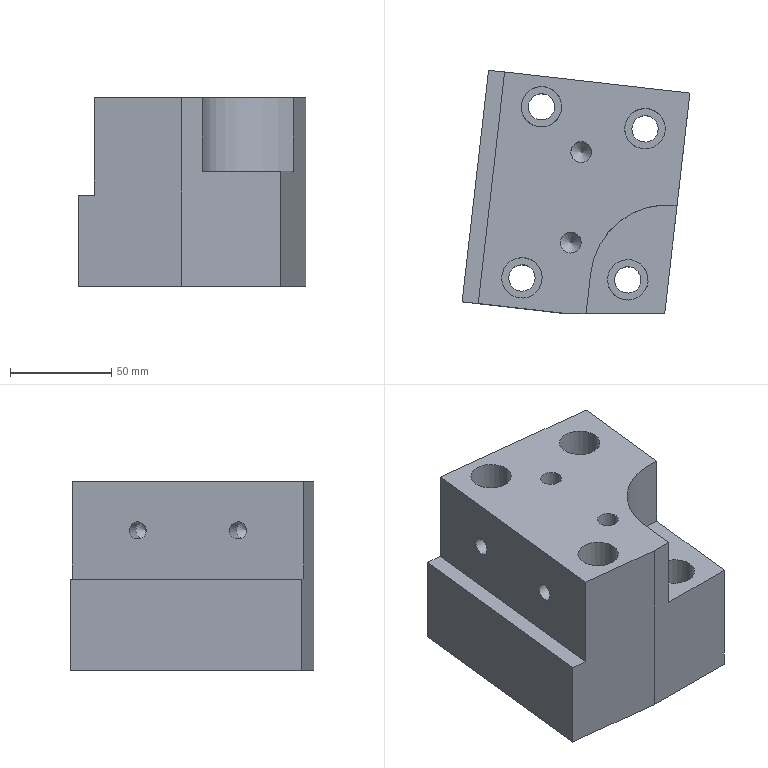Part | NX | features solid 2 | 1 solid | 32 faces | box 112.376 x 120.08 x 93 mm | volume 865745 mm3 | plane 15 | cylinder 13 | cone 4 | commonest cylinder face diameters 13 x4 20 x4 8.5 x2 10.3 x2 76 x1
STEP:
#1=CARTESIAN_POINT('',(3534.734,-298.002,-128.));
#2=VERTEX_POINT('',#1);
#3=CARTESIAN_POINT('',(3540.966,-299.848,-128.));
#4=DIRECTION('',(0.,0.,1.));
#5=DIRECTION('',(-0.9588,0.284,0.));
#6=AXIS2_PLACEMENT_3D('',#3,#4,#5);
#7=CIRCLE('',#6,6.5);
#8=EDGE_CURVE('',#2,#2,#7,.T.);
#9=ORIENTED_EDGE('',*,*,#8,.T.);
#10=EDGE_LOOP('',(#9));
#11=FACE_BOUND('',#10,.T.);
#12=CARTESIAN_POINT('',(3526.244,-372.52,-128.));
#13=VERTEX_POINT('',#12);
#14=CARTESIAN_POINT('',(3532.476,-374.366,-128.));
#15=DIRECTION('',(0.,0.,-1.));
#16=DIRECTION('',(-0.9588,0.284,0.));
#17=AXIS2_PLACEMENT_3D('',#14,#15,#16);
#18=CIRCLE('',#17,6.5);
#19=EDGE_CURVE('',#13,#13,#18,.T.);
#20=ORIENTED_EDGE('',*,*,#19,.F.);
#21=EDGE_LOOP('',(#20));
#22=FACE_BOUND('',#21,.T.);
#23=CARTESIAN_POINT('',(3474.012,-371.601,-128.));
#24=VERTEX_POINT('',#23);
#25=CARTESIAN_POINT('',(3480.244,-373.447,-128.));
#26=DIRECTION('',(0.,0.,1.));
#27=DIRECTION('',(-0.9588,0.284,0.));
#28=AXIS2_PLACEMENT_3D('',#25,#26,#27);
#29=CIRCLE('',#28,6.5);
#30=EDGE_CURVE('',#24,#24,#29,.T.);
#31=ORIENTED_EDGE('',*,*,#30,.T.);
#32=EDGE_LOOP('',(#31));
#33=FACE_BOUND('',#32,.T.);
#34=CARTESIAN_POINT('',(3483.634,-287.147,-128.));
#35=VERTEX_POINT('',#34);
#36=CARTESIAN_POINT('',(3489.867,-288.994,-128.));
#37=DIRECTION('',(0.,0.,-1.));
#38=DIRECTION('',(-0.9588,0.284,0.));
#39=AXIS2_PLACEMENT_3D('',#36,#37,#38);
#40=CIRCLE('',#39,6.5);
#41=EDGE_CURVE('',#35,#35,#40,.T.);
#42=ORIENTED_EDGE('',*,*,#41,.F.);
#43=EDGE_LOOP('',(#42));
#44=FACE_BOUND('',#43,.T.);
#45=CARTESIAN_POINT('',(3550.71,-391.,-128.));
#46=VERTEX_POINT('',#45);
#47=CARTESIAN_POINT('',(3563.102,-282.241,-128.));
#48=VERTEX_POINT('',#47);
#49=CARTESIAN_POINT('',(3549.214,-404.131,-128.));
#50=DIRECTION('',(0.1132,0.9936,0.));
#51=VECTOR('',#50,1000.);
#52=LINE('',#49,#51);
#53=EDGE_CURVE('',#46,#48,#52,.T.);
#54=ORIENTED_EDGE('',*,*,#53,.F.);
#55=CARTESIAN_POINT('',(3501.799,-391.,-128.));
#56=VERTEX_POINT('',#55);
#57=CARTESIAN_POINT('',(2433.139,-391.,-128.));
#58=DIRECTION('',(-1.,0.,0.));
#59=VECTOR('',#58,1000.);
#60=LINE('',#57,#59);
#61=EDGE_CURVE('',#46,#56,#60,.T.);
#62=ORIENTED_EDGE('',*,*,#61,.T.);
#63=CARTESIAN_POINT('',(3450.726,-385.181,-128.));
#64=VERTEX_POINT('',#63);
#65=CARTESIAN_POINT('',(3304.282,-368.496,-128.));
#66=DIRECTION('',(-0.9936,0.1132,0.));
#67=VECTOR('',#66,1000.);
#68=LINE('',#65,#67);
#69=EDGE_CURVE('',#56,#64,#68,.T.);
#70=ORIENTED_EDGE('',*,*,#69,.T.);
#71=CARTESIAN_POINT('',(3463.745,-270.92,-128.));
#72=VERTEX_POINT('',#71);
#73=CARTESIAN_POINT('',(3449.857,-392.811,-128.));
#74=DIRECTION('',(0.1132,0.9936,0.));
#75=VECTOR('',#74,1000.);
#76=LINE('',#73,#75);
#77=EDGE_CURVE('',#64,#72,#76,.T.);
#78=ORIENTED_EDGE('',*,*,#77,.T.);
#79=CARTESIAN_POINT('',(3414.066,-265.26,-128.));
#80=DIRECTION('',(0.9936,-0.1132,0.));
#81=VECTOR('',#80,1000.);
#82=LINE('',#79,#81);
#83=EDGE_CURVE('',#72,#48,#82,.T.);
#84=ORIENTED_EDGE('',*,*,#83,.T.);
#85=EDGE_LOOP('',(#54,#62,#70,#78,#84));
#86=FACE_BOUND('',#85,.T.);
#87=CARTESIAN_POINT('',(2433.139,-154.013,-128.));
#88=DIRECTION('',(0.,0.,-1.));
#89=DIRECTION('',(-0.9588,0.284,0.));
#90=AXIS2_PLACEMENT_3D('',#87,#88,#89);
#91=PLANE('',#90);
#92=ADVANCED_FACE('',(#11,#22,#33,#44,#86),#91,.T.);
#93=CARTESIAN_POINT('',(3501.799,-391.,-35.));
#94=VERTEX_POINT('',#93);
#95=CARTESIAN_POINT('',(3501.799,-391.,-118.027));
#96=DIRECTION('',(0.,0.,-1.));
#97=VECTOR('',#96,1000.);
#98=LINE('',#95,#97);
#99=EDGE_CURVE('',#94,#56,#98,.T.);
#100=ORIENTED_EDGE('',*,*,#99,.F.);
#101=CARTESIAN_POINT('',(3458.675,-386.087,-35.));
#102=VERTEX_POINT('',#101);
#103=CARTESIAN_POINT('',(3304.282,-368.496,-35.));
#104=DIRECTION('',(0.9936,-0.1132,0.));
#105=VECTOR('',#104,1000.);
#106=LINE('',#103,#105);
#107=EDGE_CURVE('',#102,#94,#106,.T.);
#108=ORIENTED_EDGE('',*,*,#107,.F.);
#109=CARTESIAN_POINT('',(3458.675,-386.087,-83.));
#110=VERTEX_POINT('',#109);
#111=CARTESIAN_POINT('',(3458.675,-386.087,-56.673));
#112=DIRECTION('',(0.,0.,1.));
#113=VECTOR('',#112,1000.);
#114=LINE('',#111,#113);
#115=EDGE_CURVE('',#110,#102,#114,.T.);
#116=ORIENTED_EDGE('',*,*,#115,.F.);
#117=CARTESIAN_POINT('',(3450.726,-385.181,-83.));
#118=VERTEX_POINT('',#117);
#119=CARTESIAN_POINT('',(3304.282,-368.496,-83.));
#120=DIRECTION('',(-0.9936,0.1132,0.));
#121=VECTOR('',#120,1000.);
#122=LINE('',#119,#121);
#123=EDGE_CURVE('',#110,#118,#122,.T.);
#124=ORIENTED_EDGE('',*,*,#123,.T.);
#125=CARTESIAN_POINT('',(3450.726,-385.181,-16.673));
#126=DIRECTION('',(0.,0.,1.));
#127=VECTOR('',#126,1000.);
#128=LINE('',#125,#127);
#129=EDGE_CURVE('',#64,#118,#128,.T.);
#130=ORIENTED_EDGE('',*,*,#129,.F.);
#131=ORIENTED_EDGE('',*,*,#69,.F.);
#132=EDGE_LOOP('',(#100,#108,#116,#124,#130,#131));
#133=FACE_BOUND('',#132,.T.);
#134=CARTESIAN_POINT('',(3304.282,-368.496,-118.027));
#135=DIRECTION('',(0.1132,0.9936,0.));
#136=DIRECTION('',(0.,0.,-1.));
#137=AXIS2_PLACEMENT_3D('',#134,#135,#136);
#138=PLANE('',#137);
#139=ADVANCED_FACE('',(#133),#138,.F.);
#140=CARTESIAN_POINT('',(3489.833,-376.287,-35.));
#141=VERTEX_POINT('',#140);
#142=CARTESIAN_POINT('',(3480.244,-373.447,-35.));
#143=DIRECTION('',(0.,0.,-1.));
#144=DIRECTION('',(0.9588,-0.284,0.));
#145=AXIS2_PLACEMENT_3D('',#142,#143,#144);
#146=CIRCLE('',#145,10.);
#147=EDGE_CURVE('',#141,#141,#146,.T.);
#148=ORIENTED_EDGE('',*,*,#147,.T.);
#149=EDGE_LOOP('',(#148));
#150=FACE_BOUND('',#149,.T.);
#151=CARTESIAN_POINT('',(3514.578,-311.938,-35.));
#152=VERTEX_POINT('',#151);
#153=CARTESIAN_POINT('',(3509.461,-311.355,-35.));
#154=DIRECTION('',(0.,0.,1.));
#155=DIRECTION('',(0.9936,-0.1132,0.));
#156=AXIS2_PLACEMENT_3D('',#153,#154,#155);
#157=CIRCLE('',#156,5.15);
#158=EDGE_CURVE('',#152,#152,#157,.T.);
#159=ORIENTED_EDGE('',*,*,#158,.F.);
#160=EDGE_LOOP('',(#159));
#161=FACE_BOUND('',#160,.T.);
#162=CARTESIAN_POINT('',(3509.484,-356.649,-35.));
#163=VERTEX_POINT('',#162);
#164=CARTESIAN_POINT('',(3504.367,-356.066,-35.));
#165=DIRECTION('',(0.,0.,1.));
#166=DIRECTION('',(0.9936,-0.1132,0.));
#167=AXIS2_PLACEMENT_3D('',#164,#165,#166);
#168=CIRCLE('',#167,5.15);
#169=EDGE_CURVE('',#163,#163,#168,.T.);
#170=ORIENTED_EDGE('',*,*,#169,.F.);
#171=EDGE_LOOP('',(#170));
#172=FACE_BOUND('',#171,.T.);
#173=CARTESIAN_POINT('',(3499.802,-290.126,-35.));
#174=VERTEX_POINT('',#173);
#175=CARTESIAN_POINT('',(3489.867,-288.994,-35.));
#176=DIRECTION('',(0.,0.,1.));
#177=DIRECTION('',(0.9936,-0.1132,0.));
#178=AXIS2_PLACEMENT_3D('',#175,#176,#177);
#179=CIRCLE('',#178,10.);
#180=EDGE_CURVE('',#174,#174,#179,.T.);
#181=ORIENTED_EDGE('',*,*,#180,.F.);
#182=EDGE_LOOP('',(#181));
#183=FACE_BOUND('',#182,.T.);
#184=CARTESIAN_POINT('',(3550.902,-300.98,-35.));
#185=VERTEX_POINT('',#184);
#186=CARTESIAN_POINT('',(3540.966,-299.848,-35.));
#187=DIRECTION('',(0.,0.,1.));
#188=DIRECTION('',(0.9936,-0.1132,0.));
#189=AXIS2_PLACEMENT_3D('',#186,#187,#188);
#190=CIRCLE('',#189,10.);
#191=EDGE_CURVE('',#185,#185,#190,.T.);
#192=ORIENTED_EDGE('',*,*,#191,.F.);
#193=EDGE_LOOP('',(#192));
#194=FACE_BOUND('',#193,.T.);
#195=ORIENTED_EDGE('',*,*,#107,.T.);
#196=CARTESIAN_POINT('',(3511.886,-391.,-35.));
#197=VERTEX_POINT('',#196);
#198=CARTESIAN_POINT('',(3507.763,-391.,-35.));
#199=DIRECTION('',(1.,0.,0.));
#200=VECTOR('',#199,1000.);
#201=LINE('',#198,#200);
#202=EDGE_CURVE('',#94,#197,#201,.T.);
#203=ORIENTED_EDGE('',*,*,#202,.T.);
#204=CARTESIAN_POINT('',(3514.147,-371.156,-35.));
#205=VERTEX_POINT('',#204);
#206=CARTESIAN_POINT('',(3519.115,-327.552,-35.));
#207=DIRECTION('',(-0.1132,-0.9936,0.));
#208=VECTOR('',#207,1000.);
#209=LINE('',#206,#208);
#210=EDGE_CURVE('',#205,#197,#209,.T.);
#211=ORIENTED_EDGE('',*,*,#210,.F.);
#212=CARTESIAN_POINT('',(3556.775,-337.771,-35.));
#213=VERTEX_POINT('',#212);
#214=CARTESIAN_POINT('',(3551.903,-375.457,-35.));
#215=DIRECTION('',(0.,0.,-1.));
#216=DIRECTION('',(0.9936,-0.1132,0.));
#217=AXIS2_PLACEMENT_3D('',#214,#215,#216);
#218=CIRCLE('',#217,38.);
#219=EDGE_CURVE('',#205,#213,#218,.T.);
#220=ORIENTED_EDGE('',*,*,#219,.T.);
#221=CARTESIAN_POINT('',(3563.102,-282.241,-35.));
#222=VERTEX_POINT('',#221);
#223=CARTESIAN_POINT('',(3549.214,-404.131,-35.));
#224=DIRECTION('',(-0.1132,-0.9936,0.));
#225=VECTOR('',#224,1000.);
#226=LINE('',#223,#225);
#227=EDGE_CURVE('',#222,#213,#226,.T.);
#228=ORIENTED_EDGE('',*,*,#227,.F.);
#229=CARTESIAN_POINT('',(3471.693,-271.826,-35.));
#230=VERTEX_POINT('',#229);
#231=CARTESIAN_POINT('',(3513.423,-276.58,-35.));
#232=DIRECTION('',(0.9936,-0.1132,0.));
#233=VECTOR('',#232,1000.);
#234=LINE('',#231,#233);
#235=EDGE_CURVE('',#230,#222,#234,.T.);
#236=ORIENTED_EDGE('',*,*,#235,.F.);
#237=CARTESIAN_POINT('',(3457.806,-393.716,-35.));
#238=DIRECTION('',(-0.1132,-0.9936,0.));
#239=VECTOR('',#238,1000.);
#240=LINE('',#237,#239);
#241=EDGE_CURVE('',#230,#102,#240,.T.);
#242=ORIENTED_EDGE('',*,*,#241,.T.);
#243=EDGE_LOOP('',(#195,#203,#211,#220,#228,#236,#242));
#244=FACE_BOUND('',#243,.T.);
#245=CARTESIAN_POINT('',(3507.763,-326.259,-35.));
#246=DIRECTION('',(0.,0.,1.));
#247=DIRECTION('',(0.9588,-0.284,0.));
#248=AXIS2_PLACEMENT_3D('',#245,#246,#247);
#249=PLANE('',#248);
#250=ADVANCED_FACE('',(#150,#161,#172,#183,#194,#244),#249,.T.);
#251=CARTESIAN_POINT('',(3550.71,-391.,-71.235));
#252=VERTEX_POINT('',#251);
#253=CARTESIAN_POINT('',(3556.775,-337.771,-71.235));
#254=VERTEX_POINT('',#253);
#255=CARTESIAN_POINT('',(3549.214,-404.131,-71.235));
#256=DIRECTION('',(0.1132,0.9936,0.));
#257=VECTOR('',#256,1000.);
#258=LINE('',#255,#257);
#259=EDGE_CURVE('',#252,#254,#258,.T.);
#260=ORIENTED_EDGE('',*,*,#259,.F.);
#261=CARTESIAN_POINT('',(3550.71,-391.,-16.673));
#262=DIRECTION('',(0.,0.,-1.));
#263=VECTOR('',#262,1000.);
#264=LINE('',#261,#263);
#265=EDGE_CURVE('',#252,#46,#264,.T.);
#266=ORIENTED_EDGE('',*,*,#265,.T.);
#267=ORIENTED_EDGE('',*,*,#53,.T.);
#268=CARTESIAN_POINT('',(3563.102,-282.241,-16.673));
#269=DIRECTION('',(0.,0.,-1.));
#270=VECTOR('',#269,1000.);
#271=LINE('',#268,#270);
#272=EDGE_CURVE('',#222,#48,#271,.T.);
#273=ORIENTED_EDGE('',*,*,#272,.F.);
#274=ORIENTED_EDGE('',*,*,#227,.T.);
#275=CARTESIAN_POINT('',(3556.775,-337.771,-68.235));
#276=DIRECTION('',(0.,0.,1.));
#277=VECTOR('',#276,1000.);
#278=LINE('',#275,#277);
#279=EDGE_CURVE('',#254,#213,#278,.T.);
#280=ORIENTED_EDGE('',*,*,#279,.F.);
#281=EDGE_LOOP('',(#260,#266,#267,#273,#274,#280));
#282=FACE_BOUND('',#281,.T.);
#283=CARTESIAN_POINT('',(3549.214,-404.131,-16.673));
#284=DIRECTION('',(0.9936,-0.1132,0.));
#285=DIRECTION('',(0.1103,0.9681,-0.225));
#286=AXIS2_PLACEMENT_3D('',#283,#284,#285);
#287=PLANE('',#286);
#288=ADVANCED_FACE('',(#282),#287,.T.);
#289=CARTESIAN_POINT('',(3511.886,-391.,-71.235));
#290=VERTEX_POINT('',#289);
#291=CARTESIAN_POINT('',(3511.886,-391.,-68.235));
#292=DIRECTION('',(0.,0.,1.));
#293=VECTOR('',#292,1000.);
#294=LINE('',#291,#293);
#295=EDGE_CURVE('',#290,#197,#294,.T.);
#296=ORIENTED_EDGE('',*,*,#295,.F.);
#297=CARTESIAN_POINT('',(3514.147,-371.156,-71.235));
#298=VERTEX_POINT('',#297);
#299=CARTESIAN_POINT('',(3514.811,-365.332,-71.235));
#300=DIRECTION('',(0.1132,0.9936,0.));
#301=VECTOR('',#300,1000.);
#302=LINE('',#299,#301);
#303=EDGE_CURVE('',#290,#298,#302,.T.);
#304=ORIENTED_EDGE('',*,*,#303,.T.);
#305=CARTESIAN_POINT('',(3514.147,-371.156,-31.618));
#306=DIRECTION('',(0.,0.,1.));
#307=VECTOR('',#306,1000.);
#308=LINE('',#305,#307);
#309=EDGE_CURVE('',#298,#205,#308,.T.);
#310=ORIENTED_EDGE('',*,*,#309,.T.);
#311=ORIENTED_EDGE('',*,*,#210,.T.);
#312=EDGE_LOOP('',(#296,#304,#310,#311));
#313=FACE_BOUND('',#312,.T.);
#314=CARTESIAN_POINT('',(3514.811,-365.332,-68.235));
#315=DIRECTION('',(-0.9936,0.1132,0.));
#316=DIRECTION('',(0.,0.,-1.));
#317=AXIS2_PLACEMENT_3D('',#314,#315,#316);
#318=PLANE('',#317);
#319=ADVANCED_FACE('',(#313),#318,.F.);
#320=CARTESIAN_POINT('',(3522.54,-373.234,-71.235));
#321=VERTEX_POINT('',#320);
#322=CARTESIAN_POINT('',(3532.476,-374.366,-71.235));
#323=DIRECTION('',(0.,0.,1.));
#324=DIRECTION('',(-0.9936,0.1132,0.));
#325=AXIS2_PLACEMENT_3D('',#322,#323,#324);
#326=CIRCLE('',#325,10.);
#327=EDGE_CURVE('',#321,#321,#326,.T.);
#328=ORIENTED_EDGE('',*,*,#327,.F.);
#329=EDGE_LOOP('',(#328));
#330=FACE_BOUND('',#329,.T.);
#331=CARTESIAN_POINT('',(3542.77,-391.,-71.235));
#332=DIRECTION('',(-1.,0.,0.));
#333=VECTOR('',#332,1000.);
#334=LINE('',#331,#333);
#335=EDGE_CURVE('',#252,#290,#334,.T.);
#336=ORIENTED_EDGE('',*,*,#335,.F.);
#337=ORIENTED_EDGE('',*,*,#259,.T.);
#338=CARTESIAN_POINT('',(3551.903,-375.457,-71.235));
#339=DIRECTION('',(0.,0.,1.));
#340=DIRECTION('',(-0.9936,0.1132,0.));
#341=AXIS2_PLACEMENT_3D('',#338,#339,#340);
#342=CIRCLE('',#341,38.);
#343=EDGE_CURVE('',#254,#298,#342,.T.);
#344=ORIENTED_EDGE('',*,*,#343,.T.);
#345=ORIENTED_EDGE('',*,*,#303,.F.);
#346=EDGE_LOOP('',(#336,#337,#344,#345));
#347=FACE_BOUND('',#346,.T.);
#348=CARTESIAN_POINT('',(3542.77,-368.517,-71.235));
#349=DIRECTION('',(0.,0.,-1.));
#350=DIRECTION('',(0.9936,-0.1132,0.));
#351=AXIS2_PLACEMENT_3D('',#348,#349,#350);
#352=PLANE('',#351);
#353=ADVANCED_FACE('',(#330,#347),#352,.F.);
#354=CARTESIAN_POINT('',(3468.069,-303.639,-63.223));
#355=VERTEX_POINT('',#354);
#356=CARTESIAN_POINT('',(3468.014,-304.117,-59.));
#357=DIRECTION('',(0.9936,-0.1132,0.));
#358=DIRECTION('',(0.01281,0.1125,-0.9936));
#359=AXIS2_PLACEMENT_3D('',#356,#357,#358);
#360=CIRCLE('',#359,4.25);
#361=EDGE_CURVE('',#355,#355,#360,.T.);
#362=ORIENTED_EDGE('',*,*,#361,.T.);
#363=EDGE_LOOP('',(#362));
#364=FACE_BOUND('',#363,.T.);
#365=CARTESIAN_POINT('',(3462.409,-353.318,-63.223));
#366=VERTEX_POINT('',#365);
#367=CARTESIAN_POINT('',(3462.354,-353.796,-59.));
#368=DIRECTION('',(0.9936,-0.1132,0.));
#369=DIRECTION('',(0.01281,0.1125,-0.9936));
#370=AXIS2_PLACEMENT_3D('',#367,#368,#369);
#371=CIRCLE('',#370,4.25);
#372=EDGE_CURVE('',#366,#366,#371,.T.);
#373=ORIENTED_EDGE('',*,*,#372,.T.);
#374=EDGE_LOOP('',(#373));
#375=FACE_BOUND('',#374,.T.);
#376=ORIENTED_EDGE('',*,*,#241,.F.);
#377=CARTESIAN_POINT('',(3471.693,-271.826,-83.));
#378=VERTEX_POINT('',#377);
#379=CARTESIAN_POINT('',(3471.693,-271.826,-56.673));
#380=DIRECTION('',(0.,0.,-1.));
#381=VECTOR('',#380,1000.);
#382=LINE('',#379,#381);
#383=EDGE_CURVE('',#230,#378,#382,.T.);
#384=ORIENTED_EDGE('',*,*,#383,.T.);
#385=CARTESIAN_POINT('',(3457.806,-393.716,-83.));
#386=DIRECTION('',(0.1132,0.9936,0.));
#387=VECTOR('',#386,1000.);
#388=LINE('',#385,#387);
#389=EDGE_CURVE('',#110,#378,#388,.T.);
#390=ORIENTED_EDGE('',*,*,#389,.F.);
#391=ORIENTED_EDGE('',*,*,#115,.T.);
#392=EDGE_LOOP('',(#376,#384,#390,#391));
#393=FACE_BOUND('',#392,.T.);
#394=CARTESIAN_POINT('',(3457.806,-393.716,-56.673));
#395=DIRECTION('',(0.9936,-0.1132,0.));
#396=DIRECTION('',(0.1103,0.9681,-0.225));
#397=AXIS2_PLACEMENT_3D('',#394,#395,#396);
#398=PLANE('',#397);
#399=ADVANCED_FACE('',(#364,#375,#393),#398,.F.);
#400=CARTESIAN_POINT('',(3470.656,-370.607,-74.447));
#401=VERTEX_POINT('',#400);
#402=CARTESIAN_POINT('',(3480.244,-373.447,-74.447));
#403=DIRECTION('',(0.,0.,-1.));
#404=DIRECTION('',(-0.9588,0.284,0.));
#405=AXIS2_PLACEMENT_3D('',#402,#403,#404);
#406=CIRCLE('',#405,10.);
#407=EDGE_CURVE('',#401,#401,#406,.T.);
#408=ORIENTED_EDGE('',*,*,#407,.T.);
#409=EDGE_LOOP('',(#408));
#410=FACE_BOUND('',#409,.T.);
#411=ORIENTED_EDGE('',*,*,#147,.F.);
#412=EDGE_LOOP('',(#411));
#413=FACE_BOUND('',#412,.T.);
#414=CARTESIAN_POINT('',(3480.244,-373.447,-61.447));
#415=DIRECTION('',(0.,0.,-1.));
#416=DIRECTION('',(-0.9588,0.284,0.));
#417=AXIS2_PLACEMENT_3D('',#414,#415,#416);
#418=CYLINDRICAL_SURFACE('',#417,10.);
#419=ADVANCED_FACE('',(#410,#413),#418,.F.);
#420=ORIENTED_EDGE('',*,*,#383,.F.);
#421=ORIENTED_EDGE('',*,*,#235,.T.);
#422=ORIENTED_EDGE('',*,*,#272,.T.);
#423=ORIENTED_EDGE('',*,*,#83,.F.);
#424=CARTESIAN_POINT('',(3463.745,-270.92,-83.));
#425=VERTEX_POINT('',#424);
#426=CARTESIAN_POINT('',(3463.745,-270.92,-16.673));
#427=DIRECTION('',(0.,0.,-1.));
#428=VECTOR('',#427,1000.);
#429=LINE('',#426,#428);
#430=EDGE_CURVE('',#425,#72,#429,.T.);
#431=ORIENTED_EDGE('',*,*,#430,.F.);
#432=CARTESIAN_POINT('',(3414.066,-265.26,-83.));
#433=DIRECTION('',(-0.9936,0.1132,0.));
#434=VECTOR('',#433,1000.);
#435=LINE('',#432,#434);
#436=EDGE_CURVE('',#378,#425,#435,.T.);
#437=ORIENTED_EDGE('',*,*,#436,.F.);
#438=EDGE_LOOP('',(#420,#421,#422,#423,#431,#437));
#439=FACE_BOUND('',#438,.T.);
#440=CARTESIAN_POINT('',(3414.066,-265.26,-45.696));
#441=DIRECTION('',(0.1132,0.9936,0.));
#442=DIRECTION('',(0.,0.,-1.));
#443=AXIS2_PLACEMENT_3D('',#440,#441,#442);
#444=PLANE('',#443);
#445=ADVANCED_FACE('',(#439),#444,.T.);
#446=ORIENTED_EDGE('',*,*,#129,.T.);
#447=CARTESIAN_POINT('',(3448.745,-402.569,-83.));
#448=DIRECTION('',(-0.1132,-0.9936,0.));
#449=VECTOR('',#448,1000.);
#450=LINE('',#447,#449);
#451=EDGE_CURVE('',#425,#118,#450,.T.);
#452=ORIENTED_EDGE('',*,*,#451,.F.);
#453=ORIENTED_EDGE('',*,*,#430,.T.);
#454=ORIENTED_EDGE('',*,*,#77,.F.);
#455=EDGE_LOOP('',(#446,#452,#453,#454));
#456=FACE_BOUND('',#455,.T.);
#457=CARTESIAN_POINT('',(3449.857,-392.811,-16.673));
#458=DIRECTION('',(0.9936,-0.1132,0.));
#459=DIRECTION('',(0.1103,0.9681,-0.225));
#460=AXIS2_PLACEMENT_3D('',#457,#458,#459);
#461=PLANE('',#460);
#462=ADVANCED_FACE('',(#456),#461,.F.);
#463=ORIENTED_EDGE('',*,*,#123,.F.);
#464=ORIENTED_EDGE('',*,*,#389,.T.);
#465=ORIENTED_EDGE('',*,*,#436,.T.);
#466=ORIENTED_EDGE('',*,*,#451,.T.);
#467=EDGE_LOOP('',(#463,#464,#465,#466));
#468=FACE_BOUND('',#467,.T.);
#469=CARTESIAN_POINT('',(3451.726,-402.908,-83.));
#470=DIRECTION('',(0.,0.,-1.));
#471=DIRECTION('',(-0.1132,-0.9936,0.));
#472=AXIS2_PLACEMENT_3D('',#469,#470,#471);
#473=PLANE('',#472);
#474=ADVANCED_FACE('',(#468),#473,.F.);
#475=CARTESIAN_POINT('',(3474.012,-371.601,-74.447));
#476=VERTEX_POINT('',#475);
#477=CARTESIAN_POINT('',(3480.244,-373.447,-74.447));
#478=DIRECTION('',(0.,0.,-1.));
#479=DIRECTION('',(-0.9588,0.284,0.));
#480=AXIS2_PLACEMENT_3D('',#477,#478,#479);
#481=CIRCLE('',#480,6.5);
#482=EDGE_CURVE('',#476,#476,#481,.T.);
#483=ORIENTED_EDGE('',*,*,#482,.F.);
#484=EDGE_LOOP('',(#483));
#485=FACE_BOUND('',#484,.T.);
#486=ORIENTED_EDGE('',*,*,#30,.F.);
#487=EDGE_LOOP('',(#486));
#488=FACE_BOUND('',#487,.T.);
#489=CARTESIAN_POINT('',(3480.244,-373.447,-61.447));
#490=DIRECTION('',(0.,0.,-1.));
#491=DIRECTION('',(-0.9588,0.284,0.));
#492=AXIS2_PLACEMENT_3D('',#489,#490,#491);
#493=CYLINDRICAL_SURFACE('',#492,6.5);
#494=ADVANCED_FACE('',(#485,#488),#493,.F.);
#495=ORIENTED_EDGE('',*,*,#482,.T.);
#496=EDGE_LOOP('',(#495));
#497=FACE_BOUND('',#496,.T.);
#498=ORIENTED_EDGE('',*,*,#407,.F.);
#499=EDGE_LOOP('',(#498));
#500=FACE_BOUND('',#499,.T.);
#501=CARTESIAN_POINT('',(3480.81,-368.479,-74.447));
#502=DIRECTION('',(0.,0.,-1.));
#503=DIRECTION('',(0.9588,-0.284,0.));
#504=AXIS2_PLACEMENT_3D('',#501,#502,#503);
#505=PLANE('',#504);
#506=ADVANCED_FACE('',(#497,#500),#505,.F.);
#507=CARTESIAN_POINT('',(3480.279,-286.153,-74.447));
#508=VERTEX_POINT('',#507);
#509=CARTESIAN_POINT('',(3489.867,-288.994,-74.447));
#510=DIRECTION('',(0.,0.,1.));
#511=DIRECTION('',(-0.9588,0.284,0.));
#512=AXIS2_PLACEMENT_3D('',#509,#510,#511);
#513=CIRCLE('',#512,10.);
#514=EDGE_CURVE('',#508,#508,#513,.T.);
#515=ORIENTED_EDGE('',*,*,#514,.F.);
#516=EDGE_LOOP('',(#515));
#517=FACE_BOUND('',#516,.T.);
#518=ORIENTED_EDGE('',*,*,#180,.T.);
#519=EDGE_LOOP('',(#518));
#520=FACE_BOUND('',#519,.T.);
#521=CARTESIAN_POINT('',(3489.867,-288.994,-61.447));
#522=DIRECTION('',(0.,0.,-1.));
#523=DIRECTION('',(-0.9981,-0.06105,0.));
#524=AXIS2_PLACEMENT_3D('',#521,#522,#523);
#525=CYLINDRICAL_SURFACE('',#524,10.);
#526=ADVANCED_FACE('',(#517,#520),#525,.F.);
#527=CARTESIAN_POINT('',(3483.634,-287.147,-74.447));
#528=VERTEX_POINT('',#527);
#529=CARTESIAN_POINT('',(3489.867,-288.994,-74.447));
#530=DIRECTION('',(0.,0.,1.));
#531=DIRECTION('',(-0.9588,0.284,0.));
#532=AXIS2_PLACEMENT_3D('',#529,#530,#531);
#533=CIRCLE('',#532,6.5);
#534=EDGE_CURVE('',#528,#528,#533,.T.);
#535=ORIENTED_EDGE('',*,*,#534,.T.);
#536=EDGE_LOOP('',(#535));
#537=FACE_BOUND('',#536,.T.);
#538=ORIENTED_EDGE('',*,*,#41,.T.);
#539=EDGE_LOOP('',(#538));
#540=FACE_BOUND('',#539,.T.);
#541=CARTESIAN_POINT('',(3489.867,-288.994,-61.447));
#542=DIRECTION('',(0.,0.,-1.));
#543=DIRECTION('',(-0.9981,-0.06105,0.));
#544=AXIS2_PLACEMENT_3D('',#541,#542,#543);
#545=CYLINDRICAL_SURFACE('',#544,6.5);
#546=ADVANCED_FACE('',(#537,#540),#545,.F.);
#547=ORIENTED_EDGE('',*,*,#534,.F.);
#548=EDGE_LOOP('',(#547));
#549=FACE_BOUND('',#548,.T.);
#550=ORIENTED_EDGE('',*,*,#514,.T.);
#551=EDGE_LOOP('',(#550));
#552=FACE_BOUND('',#551,.T.);
#553=CARTESIAN_POINT('',(3489.301,-293.961,-74.447));
#554=DIRECTION('',(0.,0.,-1.));
#555=DIRECTION('',(0.9981,0.06105,0.));
#556=AXIS2_PLACEMENT_3D('',#553,#554,#555);
#557=PLANE('',#556);
#558=ADVANCED_FACE('',(#549,#552),#557,.F.);
#559=CARTESIAN_POINT('',(3534.734,-298.002,-89.447));
#560=VERTEX_POINT('',#559);
#561=CARTESIAN_POINT('',(3540.966,-299.848,-89.447));
#562=DIRECTION('',(0.,0.,-1.));
#563=DIRECTION('',(-0.9588,0.284,0.));
#564=AXIS2_PLACEMENT_3D('',#561,#562,#563);
#565=CIRCLE('',#564,6.5);
#566=EDGE_CURVE('',#560,#560,#565,.T.);
#567=ORIENTED_EDGE('',*,*,#566,.T.);
#568=EDGE_LOOP('',(#567));
#569=FACE_BOUND('',#568,.T.);
#570=CARTESIAN_POINT('',(3531.378,-297.008,-89.447));
#571=VERTEX_POINT('',#570);
#572=CARTESIAN_POINT('',(3540.966,-299.848,-89.447));
#573=DIRECTION('',(0.,0.,-1.));
#574=DIRECTION('',(-0.9588,0.284,0.));
#575=AXIS2_PLACEMENT_3D('',#572,#573,#574);
#576=CIRCLE('',#575,10.);
#577=EDGE_CURVE('',#571,#571,#576,.T.);
#578=ORIENTED_EDGE('',*,*,#577,.F.);
#579=EDGE_LOOP('',(#578));
#580=FACE_BOUND('',#579,.T.);
#581=CARTESIAN_POINT('',(3540.966,-299.848,-89.447));
#582=DIRECTION('',(0.,0.,-1.));
#583=DIRECTION('',(-0.9588,0.284,0.));
#584=AXIS2_PLACEMENT_3D('',#581,#582,#583);
#585=PLANE('',#584);
#586=ADVANCED_FACE('',(#569,#580),#585,.F.);
#587=CARTESIAN_POINT('',(3526.244,-372.52,-89.447));
#588=VERTEX_POINT('',#587);
#589=CARTESIAN_POINT('',(3532.476,-374.366,-89.447));
#590=DIRECTION('',(0.,0.,1.));
#591=DIRECTION('',(-0.9588,0.284,0.));
#592=AXIS2_PLACEMENT_3D('',#589,#590,#591);
#593=CIRCLE('',#592,6.5);
#594=EDGE_CURVE('',#588,#588,#593,.T.);
#595=ORIENTED_EDGE('',*,*,#594,.F.);
#596=EDGE_LOOP('',(#595));
#597=FACE_BOUND('',#596,.T.);
#598=CARTESIAN_POINT('',(3522.888,-371.526,-89.447));
#599=VERTEX_POINT('',#598);
#600=CARTESIAN_POINT('',(3532.476,-374.366,-89.447));
#601=DIRECTION('',(0.,0.,1.));
#602=DIRECTION('',(-0.9588,0.284,0.));
#603=AXIS2_PLACEMENT_3D('',#600,#601,#602);
#604=CIRCLE('',#603,10.);
#605=EDGE_CURVE('',#599,#599,#604,.T.);
#606=ORIENTED_EDGE('',*,*,#605,.T.);
#607=EDGE_LOOP('',(#606));
#608=FACE_BOUND('',#607,.T.);
#609=CARTESIAN_POINT('',(3532.476,-374.366,-89.447));
#610=DIRECTION('',(0.,0.,-1.));
#611=DIRECTION('',(-0.9981,-0.06105,0.));
#612=AXIS2_PLACEMENT_3D('',#609,#610,#611);
#613=PLANE('',#612);
#614=ADVANCED_FACE('',(#597,#608),#613,.F.);
#615=ORIENTED_EDGE('',*,*,#577,.T.);
#616=EDGE_LOOP('',(#615));
#617=FACE_BOUND('',#616,.T.);
#618=ORIENTED_EDGE('',*,*,#191,.T.);
#619=EDGE_LOOP('',(#618));
#620=FACE_BOUND('',#619,.T.);
#621=CARTESIAN_POINT('',(3540.966,-299.848,-61.447));
#622=DIRECTION('',(0.,0.,-1.));
#623=DIRECTION('',(0.9588,-0.284,0.));
#624=AXIS2_PLACEMENT_3D('',#621,#622,#623);
#625=CYLINDRICAL_SURFACE('',#624,10.);
#626=ADVANCED_FACE('',(#617,#620),#625,.F.);
#627=ORIENTED_EDGE('',*,*,#566,.F.);
#628=EDGE_LOOP('',(#627));
#629=FACE_BOUND('',#628,.T.);
#630=ORIENTED_EDGE('',*,*,#8,.F.);
#631=EDGE_LOOP('',(#630));
#632=FACE_BOUND('',#631,.T.);
#633=CARTESIAN_POINT('',(3540.966,-299.848,-61.447));
#634=DIRECTION('',(0.,0.,-1.));
#635=DIRECTION('',(0.9588,-0.284,0.));
#636=AXIS2_PLACEMENT_3D('',#633,#634,#635);
#637=CYLINDRICAL_SURFACE('',#636,6.5);
#638=ADVANCED_FACE('',(#629,#632),#637,.F.);
#639=ORIENTED_EDGE('',*,*,#594,.T.);
#640=EDGE_LOOP('',(#639));
#641=FACE_BOUND('',#640,.T.);
#642=ORIENTED_EDGE('',*,*,#19,.T.);
#643=EDGE_LOOP('',(#642));
#644=FACE_BOUND('',#643,.T.);
#645=CARTESIAN_POINT('',(3532.476,-374.366,-61.447));
#646=DIRECTION('',(0.,0.,-1.));
#647=DIRECTION('',(0.9981,0.06105,0.));
#648=AXIS2_PLACEMENT_3D('',#645,#646,#647);
#649=CYLINDRICAL_SURFACE('',#648,6.5);
#650=ADVANCED_FACE('',(#641,#644),#649,.F.);
#651=ORIENTED_EDGE('',*,*,#327,.T.);
#652=EDGE_LOOP('',(#651));
#653=FACE_BOUND('',#652,.T.);
#654=ORIENTED_EDGE('',*,*,#605,.F.);
#655=EDGE_LOOP('',(#654));
#656=FACE_BOUND('',#655,.T.);
#657=CARTESIAN_POINT('',(3532.476,-374.366,-61.447));
#658=DIRECTION('',(0.,0.,-1.));
#659=DIRECTION('',(0.9981,0.06105,0.));
#660=AXIS2_PLACEMENT_3D('',#657,#658,#659);
#661=CYLINDRICAL_SURFACE('',#660,10.);
#662=ADVANCED_FACE('',(#653,#656),#661,.F.);
#663=CARTESIAN_POINT('',(3509.461,-311.355,-69.447));
#664=VERTEX_POINT('',#663);
#665=VERTEX_LOOP('',#664);
#666=FACE_BOUND('',#665,.T.);
#667=CARTESIAN_POINT('',(3514.578,-311.938,-64.297));
#668=VERTEX_POINT('',#667);
#669=CARTESIAN_POINT('',(3509.461,-311.355,-64.297));
#670=DIRECTION('',(0.,0.,-1.));
#671=DIRECTION('',(0.9936,-0.1132,0.));
#672=AXIS2_PLACEMENT_3D('',#669,#670,#671);
#673=CIRCLE('',#672,5.15);
#674=EDGE_CURVE('',#668,#668,#673,.T.);
#675=ORIENTED_EDGE('',*,*,#674,.F.);
#676=EDGE_LOOP('',(#675));
#677=FACE_BOUND('',#676,.T.);
#678=CARTESIAN_POINT('',(3509.461,-311.355,-65.197));
#679=DIRECTION('',(0.,0.,1.));
#680=DIRECTION('',(0.9588,-0.284,0.));
#681=AXIS2_PLACEMENT_3D('',#678,#679,#680);
#682=CONICAL_SURFACE('',#681,4.25,0.7854);
#683=ADVANCED_FACE('',(#666,#677),#682,.F.);
#684=ORIENTED_EDGE('',*,*,#674,.T.);
#685=EDGE_LOOP('',(#684));
#686=FACE_BOUND('',#685,.T.);
#687=ORIENTED_EDGE('',*,*,#158,.T.);
#688=EDGE_LOOP('',(#687));
#689=FACE_BOUND('',#688,.T.);
#690=CARTESIAN_POINT('',(3509.461,-311.355,95.553));
#691=DIRECTION('',(0.,0.,-1.));
#692=DIRECTION('',(-0.9588,0.284,0.));
#693=AXIS2_PLACEMENT_3D('',#690,#691,#692);
#694=CYLINDRICAL_SURFACE('',#693,5.15);
#695=ADVANCED_FACE('',(#686,#689),#694,.F.);
#696=CARTESIAN_POINT('',(3502.904,-361.004,-59.297));
#697=VERTEX_POINT('',#696);
#698=CARTESIAN_POINT('',(3504.367,-356.066,-59.297));
#699=DIRECTION('',(0.,0.,-1.));
#700=DIRECTION('',(-0.284,-0.9588,0.));
#701=AXIS2_PLACEMENT_3D('',#698,#699,#700);
#702=CIRCLE('',#701,5.15);
#703=EDGE_CURVE('',#697,#697,#702,.T.);
#704=ORIENTED_EDGE('',*,*,#703,.F.);
#705=EDGE_LOOP('',(#704));
#706=FACE_BOUND('',#705,.T.);
#707=CARTESIAN_POINT('',(3504.367,-356.066,-64.447));
#708=VERTEX_POINT('',#707);
#709=VERTEX_LOOP('',#708);
#710=FACE_BOUND('',#709,.T.);
#711=CARTESIAN_POINT('',(3504.367,-356.066,-60.197));
#712=DIRECTION('',(0.,0.,1.));
#713=DIRECTION('',(-0.284,-0.9588,0.));
#714=AXIS2_PLACEMENT_3D('',#711,#712,#713);
#715=CONICAL_SURFACE('',#714,4.25,0.7854);
#716=ADVANCED_FACE('',(#706,#710),#715,.F.);
#717=ORIENTED_EDGE('',*,*,#703,.T.);
#718=EDGE_LOOP('',(#717));
#719=FACE_BOUND('',#718,.T.);
#720=ORIENTED_EDGE('',*,*,#169,.T.);
#721=EDGE_LOOP('',(#720));
#722=FACE_BOUND('',#721,.T.);
#723=CARTESIAN_POINT('',(3504.367,-356.066,95.553));
#724=DIRECTION('',(0.,0.,-1.));
#725=DIRECTION('',(-0.9981,-0.06105,0.));
#726=AXIS2_PLACEMENT_3D('',#723,#724,#725);
#727=CYLINDRICAL_SURFACE('',#726,5.15);
#728=ADVANCED_FACE('',(#719,#722),#727,.F.);
#729=ORIENTED_EDGE('',*,*,#279,.T.);
#730=ORIENTED_EDGE('',*,*,#219,.F.);
#731=ORIENTED_EDGE('',*,*,#309,.F.);
#732=ORIENTED_EDGE('',*,*,#343,.F.);
#733=EDGE_LOOP('',(#729,#730,#731,#732));
#734=FACE_BOUND('',#733,.T.);
#735=CARTESIAN_POINT('',(3551.903,-375.457,-68.235));
#736=DIRECTION('',(0.,0.,1.));
#737=DIRECTION('',(-0.9936,0.1132,0.));
#738=AXIS2_PLACEMENT_3D('',#735,#736,#737);
#739=CYLINDRICAL_SURFACE('',#738,38.);
#740=ADVANCED_FACE('',(#734),#739,.F.);
#741=ORIENTED_EDGE('',*,*,#61,.F.);
#742=ORIENTED_EDGE('',*,*,#265,.F.);
#743=ORIENTED_EDGE('',*,*,#335,.T.);
#744=ORIENTED_EDGE('',*,*,#295,.T.);
#745=ORIENTED_EDGE('',*,*,#202,.F.);
#746=ORIENTED_EDGE('',*,*,#99,.T.);
#747=EDGE_LOOP('',(#741,#742,#743,#744,#745,#746));
#748=FACE_BOUND('',#747,.T.);
#749=CARTESIAN_POINT('',(3609.,-391.,0.));
#750=DIRECTION('',(0.,-1.,0.));
#751=DIRECTION('',(-1.,0.,0.));
#752=AXIS2_PLACEMENT_3D('',#749,#750,#751);
#753=PLANE('',#752);
#754=ADVANCED_FACE('',(#748),#753,.T.);
#755=ORIENTED_EDGE('',*,*,#372,.F.);
#756=EDGE_LOOP('',(#755));
#757=FACE_BOUND('',#756,.T.);
#758=CARTESIAN_POINT('',(3492.394,-352.941,-59.));
#759=VERTEX_POINT('',#758);
#760=CARTESIAN_POINT('',(3491.913,-357.163,-59.));
#761=DIRECTION('',(0.9936,-0.1132,0.));
#762=DIRECTION('',(0.1132,0.9936,0.));
#763=AXIS2_PLACEMENT_3D('',#760,#761,#762);
#764=CIRCLE('',#763,4.25);
#765=EDGE_CURVE('',#759,#759,#764,.T.);
#766=ORIENTED_EDGE('',*,*,#765,.T.);
#767=EDGE_LOOP('',(#766));
#768=FACE_BOUND('',#767,.T.);
#769=CARTESIAN_POINT('',(3462.354,-353.796,-59.));
#770=DIRECTION('',(0.9936,-0.1132,0.));
#771=DIRECTION('',(-0.01281,-0.1125,0.9936));
#772=AXIS2_PLACEMENT_3D('',#769,#770,#771);
#773=CYLINDRICAL_SURFACE('',#772,4.25);
#774=ADVANCED_FACE('',(#757,#768),#773,.F.);
#775=CARTESIAN_POINT('',(3496.135,-357.644,-59.));
#776=VERTEX_POINT('',#775);
#777=VERTEX_LOOP('',#776);
#778=FACE_BOUND('',#777,.T.);
#779=ORIENTED_EDGE('',*,*,#765,.F.);
#780=EDGE_LOOP('',(#779));
#781=FACE_BOUND('',#780,.T.);
#782=CARTESIAN_POINT('',(3491.913,-357.163,-59.));
#783=DIRECTION('',(-0.9936,0.1132,0.));
#784=DIRECTION('',(0.1132,0.9936,0.));
#785=AXIS2_PLACEMENT_3D('',#782,#783,#784);
#786=CONICAL_SURFACE('',#785,4.25,0.7854);
#787=ADVANCED_FACE('',(#778,#781),#786,.F.);
#788=ORIENTED_EDGE('',*,*,#361,.F.);
#789=EDGE_LOOP('',(#788));
#790=FACE_BOUND('',#789,.T.);
#791=CARTESIAN_POINT('',(3498.054,-303.262,-59.));
#792=VERTEX_POINT('',#791);
#793=CARTESIAN_POINT('',(3497.573,-307.485,-59.));
#794=DIRECTION('',(0.9936,-0.1132,0.));
#795=DIRECTION('',(0.1132,0.9936,0.));
#796=AXIS2_PLACEMENT_3D('',#793,#794,#795);
#797=CIRCLE('',#796,4.25);
#798=EDGE_CURVE('',#792,#792,#797,.T.);
#799=ORIENTED_EDGE('',*,*,#798,.T.);
#800=EDGE_LOOP('',(#799));
#801=FACE_BOUND('',#800,.T.);
#802=CARTESIAN_POINT('',(3468.014,-304.117,-59.));
#803=DIRECTION('',(0.9936,-0.1132,0.));
#804=DIRECTION('',(-0.01281,-0.1125,0.9936));
#805=AXIS2_PLACEMENT_3D('',#802,#803,#804);
#806=CYLINDRICAL_SURFACE('',#805,4.25);
#807=ADVANCED_FACE('',(#790,#801),#806,.F.);
#808=CARTESIAN_POINT('',(3501.796,-307.966,-59.));
#809=VERTEX_POINT('',#808);
#810=VERTEX_LOOP('',#809);
#811=FACE_BOUND('',#810,.T.);
#812=ORIENTED_EDGE('',*,*,#798,.F.);
#813=EDGE_LOOP('',(#812));
#814=FACE_BOUND('',#813,.T.);
#815=CARTESIAN_POINT('',(3497.573,-307.485,-59.));
#816=DIRECTION('',(-0.9936,0.1132,0.));
#817=DIRECTION('',(0.1132,0.9936,0.));
#818=AXIS2_PLACEMENT_3D('',#815,#816,#817);
#819=CONICAL_SURFACE('',#818,4.25,0.7854);
#820=ADVANCED_FACE('',(#811,#814),#819,.F.);
#821=CLOSED_SHELL('',(#92,#139,#250,#288,#319,#353,#399,#419,#445,#462,#474,#494,#506,#526,#546,#558,#586,#614,#626,#638,#650,#662,#683,#695,#716,#728,#740,#754,#774,#787,#807,#820));
#822=MANIFOLD_SOLID_BREP('',#821);
#823=(LENGTH_UNIT()NAMED_UNIT(*)SI_UNIT(.MILLI.,.METRE.));
#824=UNCERTAINTY_MEASURE_WITH_UNIT(LENGTH_MEASURE(0.00001),#823,'','');
#825=(NAMED_UNIT(*)PLANE_ANGLE_UNIT()SI_UNIT($,.RADIAN.));
#826=(NAMED_UNIT(*)SI_UNIT($,.STERADIAN.)SOLID_ANGLE_UNIT());
#827=(GEOMETRIC_REPRESENTATION_CONTEXT(3)GLOBAL_UNCERTAINTY_ASSIGNED_CONTEXT((#824))GLOBAL_UNIT_ASSIGNED_CONTEXT((#823,#825,#826))REPRESENTATION_CONTEXT('',''));
#828=ADVANCED_BREP_SHAPE_REPRESENTATION('',(#822),#827);